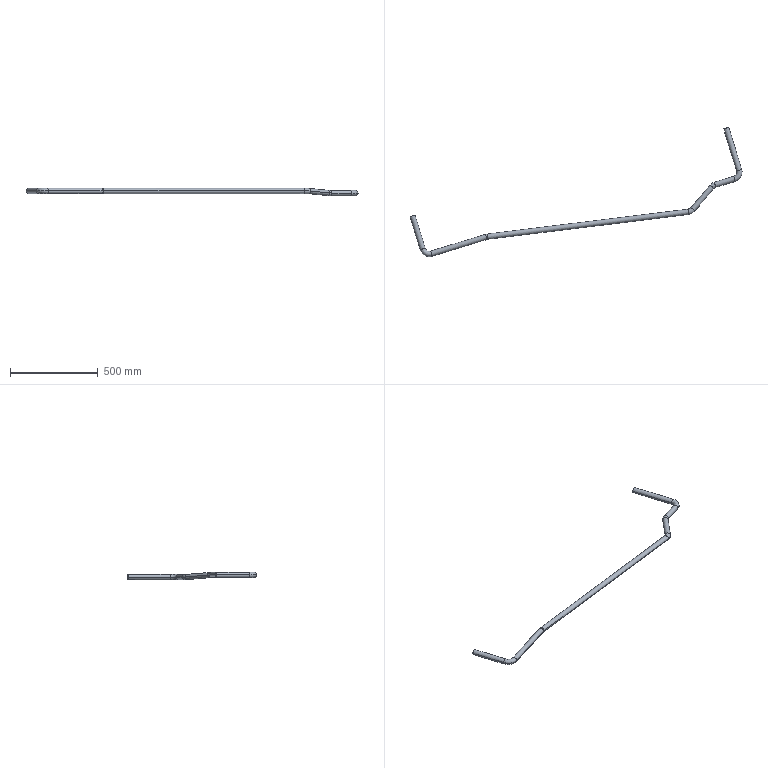Part | SolidWorks | features 3DProfileFeature 2, Sweep 1 | 1 solid | 46 faces | box 1894 x 737.142 x 42.475 mm | volume 941942 mm3 | cylinder 24 | torus 20 | plane 2 | commonest cylinder face diameters 20 x12 30 x12
STEP:
#1=CARTESIAN_POINT('',(1993.335,-11.562,-11.65));
#2=VERTEX_POINT('',#1);
#3=CARTESIAN_POINT('',(1999.193,-30.685,-11.65));
#4=VERTEX_POINT('',#3);
#5=CARTESIAN_POINT('',(1996.264,-21.124,-11.65));
#6=DIRECTION('',(-0.9561,-0.2929,0.));
#7=DIRECTION('',(-0.2929,0.9561,0.));
#8=AXIS2_PLACEMENT_3D('',#5,#6,#7);
#9=CIRCLE('',#8,10.);
#10=EDGE_CURVE('',#2,#4,#9,.T.);
#11=ORIENTED_EDGE('',*,*,#10,.T.);
#12=CARTESIAN_POINT('',(2032.355,31.767,-11.65));
#13=VERTEX_POINT('',#12);
#14=CARTESIAN_POINT('',(1984.548,17.122,-11.65));
#15=DIRECTION('',(0.,0.,1.));
#16=DIRECTION('',(0.,-1.,0.));
#17=AXIS2_PLACEMENT_3D('',#14,#15,#16);
#18=CIRCLE('',#17,50.);
#19=EDGE_CURVE('',#4,#13,#18,.T.);
#20=ORIENTED_EDGE('',*,*,#19,.T.);
#21=CARTESIAN_POINT('',(2013.232,25.909,-11.65));
#22=VERTEX_POINT('',#21);
#23=CARTESIAN_POINT('',(2022.793,28.838,-11.65));
#24=DIRECTION('',(0.2929,-0.9561,0.));
#25=DIRECTION('',(0.9561,0.2929,0.));
#26=AXIS2_PLACEMENT_3D('',#23,#24,#25);
#27=CIRCLE('',#26,10.);
#28=EDGE_CURVE('',#22,#13,#27,.T.);
#29=ORIENTED_EDGE('',*,*,#28,.F.);
#30=CARTESIAN_POINT('',(1984.548,17.122,-11.65));
#31=DIRECTION('',(0.,0.,1.));
#32=DIRECTION('',(0.,-1.,0.));
#33=AXIS2_PLACEMENT_3D('',#30,#31,#32);
#34=CIRCLE('',#33,30.);
#35=EDGE_CURVE('',#2,#22,#34,.T.);
#36=ORIENTED_EDGE('',*,*,#35,.F.);
#37=EDGE_LOOP('',(#11,#20,#29,#36));
#38=FACE_OUTER_BOUND('',#37,.T.);
#39=CARTESIAN_POINT('',(1984.548,17.122,-11.65));
#40=DIRECTION('',(0.,0.,1.));
#41=DIRECTION('',(0.,-1.,0.));
#42=AXIS2_PLACEMENT_3D('',#39,#40,#41);
#43=TOROIDAL_SURFACE('',#42,40.,10.);
#44=ADVANCED_FACE('',(#38),#43,.F.);
#45=CARTESIAN_POINT('',(1859.636,-60.808,-10.9));
#46=VERTEX_POINT('',#45);
#47=CARTESIAN_POINT('',(1859.633,-60.888,-11.886));
#48=VERTEX_POINT('',#47);
#49=CARTESIAN_POINT('',(1867.261,-67.278,-10.9));
#50=DIRECTION('',(-0.6457,-0.7609,0.06365));
#51=DIRECTION('',(-0.7625,0.647,0.));
#52=AXIS2_PLACEMENT_3D('',#49,#50,#51);
#53=CIRCLE('',#52,10.);
#54=EDGE_CURVE('',#46,#48,#53,.T.);
#55=ORIENTED_EDGE('',*,*,#54,.T.);
#56=CARTESIAN_POINT('',(1883.229,-45.365,-12.824));
#57=VERTEX_POINT('',#56);
#58=CARTESIAN_POINT('',(1897.773,-92.841,-6.953));
#59=DIRECTION('',(0.03439,-0.1123,-0.9931));
#60=DIRECTION('',(0.,0.9937,-0.1123));
#61=AXIS2_PLACEMENT_3D('',#58,#59,#60);
#62=CIRCLE('',#61,50.);
#63=EDGE_CURVE('',#48,#57,#62,.T.);
#64=ORIENTED_EDGE('',*,*,#63,.T.);
#65=CARTESIAN_POINT('',(1883.209,-45.298,-11.65));
#66=VERTEX_POINT('',#65);
#67=CARTESIAN_POINT('',(1886.138,-54.86,-11.65));
#68=DIRECTION('',(-0.9561,-0.2929,0.));
#69=DIRECTION('',(0.2929,-0.9561,0.));
#70=AXIS2_PLACEMENT_3D('',#67,#68,#69);
#71=CIRCLE('',#70,10.);
#72=EDGE_CURVE('',#66,#57,#71,.T.);
#73=ORIENTED_EDGE('',*,*,#72,.F.);
#74=CARTESIAN_POINT('',(1889.047,-64.355,-10.476));
#75=VERTEX_POINT('',#74);
#76=CARTESIAN_POINT('',(1886.138,-54.86,-11.65));
#77=DIRECTION('',(-0.9561,-0.2929,0.));
#78=DIRECTION('',(0.2929,-0.9561,0.));
#79=AXIS2_PLACEMENT_3D('',#76,#77,#78);
#80=CIRCLE('',#79,10.);
#81=EDGE_CURVE('',#75,#66,#80,.T.);
#82=ORIENTED_EDGE('',*,*,#81,.F.);
#83=CARTESIAN_POINT('',(1874.889,-73.669,-9.913));
#84=VERTEX_POINT('',#83);
#85=CARTESIAN_POINT('',(1897.773,-92.841,-6.953));
#86=DIRECTION('',(0.03439,-0.1123,-0.9931));
#87=DIRECTION('',(0.,0.9937,-0.1123));
#88=AXIS2_PLACEMENT_3D('',#85,#86,#87);
#89=CIRCLE('',#88,30.);
#90=EDGE_CURVE('',#84,#75,#89,.T.);
#91=ORIENTED_EDGE('',*,*,#90,.F.);
#92=CARTESIAN_POINT('',(1867.261,-67.278,-10.9));
#93=DIRECTION('',(-0.6457,-0.7609,0.06365));
#94=DIRECTION('',(-0.7625,0.647,0.));
#95=AXIS2_PLACEMENT_3D('',#92,#93,#94);
#96=CIRCLE('',#95,10.);
#97=EDGE_CURVE('',#84,#46,#96,.T.);
#98=ORIENTED_EDGE('',*,*,#97,.T.);
#99=EDGE_LOOP('',(#55,#64,#73,#82,#91,#98));
#100=FACE_OUTER_BOUND('',#99,.T.);
#101=CARTESIAN_POINT('',(1897.773,-92.841,-6.953));
#102=DIRECTION('',(0.03439,-0.1123,-0.9931));
#103=DIRECTION('',(0.,0.9937,-0.1123));
#104=AXIS2_PLACEMENT_3D('',#101,#102,#103);
#105=TOROIDAL_SURFACE('',#104,40.,10.);
#106=ADVANCED_FACE('',(#100),#105,.F.);
#107=CARTESIAN_POINT('',(1733.998,-219.279,0.8251));
#108=VERTEX_POINT('',#107);
#109=CARTESIAN_POINT('',(1733.992,-219.235,1.762));
#110=VERTEX_POINT('',#109);
#111=CARTESIAN_POINT('',(1732.773,-209.354,0.8251));
#112=DIRECTION('',(-0.9925,-0.1224,0.));
#113=DIRECTION('',(-0.1224,0.9925,0.));
#114=AXIS2_PLACEMENT_3D('',#111,#112,#113);
#115=CIRCLE('',#114,10.);
#116=EDGE_CURVE('',#108,#110,#115,.T.);
#117=ORIENTED_EDGE('',*,*,#116,.T.);
#118=CARTESIAN_POINT('',(1766.072,-201.937,0.5159));
#119=VERTEX_POINT('',#118);
#120=CARTESIAN_POINT('',(1727.898,-169.83,-2.924));
#121=DIRECTION('',(-0.01147,0.09302,0.9956));
#122=DIRECTION('',(0.,-0.9957,0.09303));
#123=AXIS2_PLACEMENT_3D('',#120,#121,#122);
#124=CIRCLE('',#123,50.);
#125=EDGE_CURVE('',#110,#119,#124,.T.);
#126=ORIENTED_EDGE('',*,*,#125,.T.);
#127=CARTESIAN_POINT('',(1766.062,-201.986,-0.1721));
#128=VERTEX_POINT('',#127);
#129=CARTESIAN_POINT('',(1758.438,-195.515,-0.1721));
#130=DIRECTION('',(-0.6457,-0.7609,0.06365));
#131=DIRECTION('',(0.7625,-0.647,0.));
#132=AXIS2_PLACEMENT_3D('',#129,#130,#131);
#133=CIRCLE('',#132,10.);
#134=EDGE_CURVE('',#128,#119,#133,.T.);
#135=ORIENTED_EDGE('',*,*,#134,.F.);
#136=CARTESIAN_POINT('',(1750.803,-189.094,-0.8601));
#137=VERTEX_POINT('',#136);
#138=CARTESIAN_POINT('',(1758.438,-195.515,-0.1721));
#139=DIRECTION('',(-0.6457,-0.7609,0.06365));
#140=DIRECTION('',(0.7625,-0.647,0.));
#141=AXIS2_PLACEMENT_3D('',#138,#139,#140);
#142=CIRCLE('',#141,10.);
#143=EDGE_CURVE('',#137,#128,#142,.T.);
#144=ORIENTED_EDGE('',*,*,#143,.F.);
#145=CARTESIAN_POINT('',(1731.555,-199.473,-0.1122));
#146=VERTEX_POINT('',#145);
#147=CARTESIAN_POINT('',(1727.898,-169.83,-2.924));
#148=DIRECTION('',(-0.01147,0.09302,0.9956));
#149=DIRECTION('',(0.,-0.9957,0.09303));
#150=AXIS2_PLACEMENT_3D('',#147,#148,#149);
#151=CIRCLE('',#150,30.);
#152=EDGE_CURVE('',#146,#137,#151,.T.);
#153=ORIENTED_EDGE('',*,*,#152,.F.);
#154=CARTESIAN_POINT('',(1732.773,-209.354,0.8251));
#155=DIRECTION('',(-0.9925,-0.1224,0.));
#156=DIRECTION('',(-0.1224,0.9925,0.));
#157=AXIS2_PLACEMENT_3D('',#154,#155,#156);
#158=CIRCLE('',#157,10.);
#159=EDGE_CURVE('',#146,#108,#158,.T.);
#160=ORIENTED_EDGE('',*,*,#159,.T.);
#161=EDGE_LOOP('',(#117,#126,#135,#144,#153,#160));
#162=FACE_OUTER_BOUND('',#161,.T.);
#163=CARTESIAN_POINT('',(1727.898,-169.83,-2.924));
#164=DIRECTION('',(-0.01147,0.09302,0.9956));
#165=DIRECTION('',(0.,-0.9957,0.09303));
#166=AXIS2_PLACEMENT_3D('',#163,#164,#165);
#167=TOROIDAL_SURFACE('',#166,40.,10.);
#168=ADVANCED_FACE('',(#162),#167,.F.);
#169=CARTESIAN_POINT('',(583.508,-361.652,0.8251));
#170=VERTEX_POINT('',#169);
#171=CARTESIAN_POINT('',(577.65,-342.529,0.8251));
#172=VERTEX_POINT('',#171);
#173=CARTESIAN_POINT('',(580.579,-352.09,0.8251));
#174=DIRECTION('',(-0.9561,-0.2929,0.));
#175=DIRECTION('',(-0.2929,0.9561,0.));
#176=AXIS2_PLACEMENT_3D('',#173,#174,#175);
#177=CIRCLE('',#176,10.);
#178=EDGE_CURVE('',#170,#172,#177,.T.);
#179=ORIENTED_EDGE('',*,*,#178,.T.);
#180=CARTESIAN_POINT('',(586.174,-340.712,0.8251));
#181=VERTEX_POINT('',#180);
#182=CARTESIAN_POINT('',(592.295,-390.336,0.8251));
#183=DIRECTION('',(0.,0.,-1.));
#184=DIRECTION('',(0.,1.,0.));
#185=AXIS2_PLACEMENT_3D('',#182,#183,#184);
#186=CIRCLE('',#185,50.);
#187=EDGE_CURVE('',#172,#181,#186,.T.);
#188=ORIENTED_EDGE('',*,*,#187,.T.);
#189=CARTESIAN_POINT('',(588.622,-360.561,0.8251));
#190=VERTEX_POINT('',#189);
#191=CARTESIAN_POINT('',(587.398,-350.637,0.8251));
#192=DIRECTION('',(-0.9925,-0.1224,0.));
#193=DIRECTION('',(0.1224,-0.9925,0.));
#194=AXIS2_PLACEMENT_3D('',#191,#192,#193);
#195=CIRCLE('',#194,10.);
#196=EDGE_CURVE('',#190,#181,#195,.T.);
#197=ORIENTED_EDGE('',*,*,#196,.F.);
#198=CARTESIAN_POINT('',(592.295,-390.336,0.8251));
#199=DIRECTION('',(0.,0.,-1.));
#200=DIRECTION('',(0.,1.,0.));
#201=AXIS2_PLACEMENT_3D('',#198,#199,#200);
#202=CIRCLE('',#201,30.);
#203=EDGE_CURVE('',#170,#190,#202,.T.);
#204=ORIENTED_EDGE('',*,*,#203,.F.);
#205=EDGE_LOOP('',(#179,#188,#197,#204));
#206=FACE_OUTER_BOUND('',#205,.T.);
#207=CARTESIAN_POINT('',(592.295,-390.336,0.8251));
#208=DIRECTION('',(0.,0.,-1.));
#209=DIRECTION('',(0.,1.,0.));
#210=AXIS2_PLACEMENT_3D('',#207,#208,#209);
#211=TOROIDAL_SURFACE('',#210,40.,10.);
#212=ADVANCED_FACE('',(#206),#211,.F.);
#213=CARTESIAN_POINT('',(227.44,-418.436,0.8251));
#214=VERTEX_POINT('',#213);
#215=CARTESIAN_POINT('',(208.318,-424.294,0.8251));
#216=VERTEX_POINT('',#215);
#217=CARTESIAN_POINT('',(217.879,-421.365,0.8251));
#218=DIRECTION('',(-0.2929,0.9561,0.));
#219=DIRECTION('',(0.9561,0.2929,0.));
#220=AXIS2_PLACEMENT_3D('',#217,#218,#219);
#221=CIRCLE('',#220,10.);
#222=EDGE_CURVE('',#214,#216,#221,.T.);
#223=ORIENTED_EDGE('',*,*,#222,.T.);
#224=CARTESIAN_POINT('',(270.77,-457.456,0.8251));
#225=VERTEX_POINT('',#224);
#226=CARTESIAN_POINT('',(256.125,-409.649,0.8251));
#227=DIRECTION('',(0.,0.,1.));
#228=DIRECTION('',(1.,0.,0.));
#229=AXIS2_PLACEMENT_3D('',#226,#227,#228);
#230=CIRCLE('',#229,50.);
#231=EDGE_CURVE('',#216,#225,#230,.T.);
#232=ORIENTED_EDGE('',*,*,#231,.T.);
#233=CARTESIAN_POINT('',(264.912,-438.333,0.8251));
#234=VERTEX_POINT('',#233);
#235=CARTESIAN_POINT('',(267.841,-447.894,0.8251));
#236=DIRECTION('',(-0.9561,-0.2929,0.));
#237=DIRECTION('',(0.2929,-0.9561,0.));
#238=AXIS2_PLACEMENT_3D('',#235,#236,#237);
#239=CIRCLE('',#238,10.);
#240=EDGE_CURVE('',#234,#225,#239,.T.);
#241=ORIENTED_EDGE('',*,*,#240,.F.);
#242=CARTESIAN_POINT('',(256.125,-409.649,0.8251));
#243=DIRECTION('',(0.,0.,1.));
#244=DIRECTION('',(1.,0.,0.));
#245=AXIS2_PLACEMENT_3D('',#242,#243,#244);
#246=CIRCLE('',#245,30.);
#247=EDGE_CURVE('',#214,#234,#246,.T.);
#248=ORIENTED_EDGE('',*,*,#247,.F.);
#249=EDGE_LOOP('',(#223,#232,#241,#248));
#250=FACE_OUTER_BOUND('',#249,.T.);
#251=CARTESIAN_POINT('',(256.125,-409.649,0.8251));
#252=DIRECTION('',(0.,0.,1.));
#253=DIRECTION('',(1.,0.,0.));
#254=AXIS2_PLACEMENT_3D('',#251,#252,#253);
#255=TOROIDAL_SURFACE('',#254,40.,10.);
#256=ADVANCED_FACE('',(#250),#255,.F.);
#257=CARTESIAN_POINT('',(2000.658,-35.466,-11.65));
#258=VERTEX_POINT('',#257);
#259=CARTESIAN_POINT('',(1991.87,-6.782,-11.65));
#260=VERTEX_POINT('',#259);
#261=CARTESIAN_POINT('',(1996.264,-21.124,-11.65));
#262=DIRECTION('',(-0.9561,-0.2929,0.));
#263=DIRECTION('',(0.2929,-0.9561,0.));
#264=AXIS2_PLACEMENT_3D('',#261,#262,#263);
#265=CIRCLE('',#264,15.);
#266=EDGE_CURVE('',#258,#260,#265,.T.);
#267=ORIENTED_EDGE('',*,*,#266,.F.);
#268=CARTESIAN_POINT('',(2037.136,33.232,-11.65));
#269=VERTEX_POINT('',#268);
#270=CARTESIAN_POINT('',(1984.548,17.122,-11.65));
#271=DIRECTION('',(0.,0.,1.));
#272=DIRECTION('',(0.,-1.,0.));
#273=AXIS2_PLACEMENT_3D('',#270,#271,#272);
#274=CIRCLE('',#273,55.);
#275=EDGE_CURVE('',#258,#269,#274,.T.);
#276=ORIENTED_EDGE('',*,*,#275,.T.);
#277=CARTESIAN_POINT('',(2008.451,24.445,-11.65));
#278=VERTEX_POINT('',#277);
#279=CARTESIAN_POINT('',(2022.793,28.838,-11.65));
#280=DIRECTION('',(0.2929,-0.9561,0.));
#281=DIRECTION('',(0.9561,0.2929,0.));
#282=AXIS2_PLACEMENT_3D('',#279,#280,#281);
#283=CIRCLE('',#282,15.);
#284=EDGE_CURVE('',#269,#278,#283,.T.);
#285=ORIENTED_EDGE('',*,*,#284,.T.);
#286=CARTESIAN_POINT('',(1984.548,17.122,-11.65));
#287=DIRECTION('',(0.,0.,1.));
#288=DIRECTION('',(0.,-1.,0.));
#289=AXIS2_PLACEMENT_3D('',#286,#287,#288);
#290=CIRCLE('',#289,25.);
#291=EDGE_CURVE('',#260,#278,#290,.T.);
#292=ORIENTED_EDGE('',*,*,#291,.F.);
#293=EDGE_LOOP('',(#267,#276,#285,#292));
#294=FACE_OUTER_BOUND('',#293,.T.);
#295=CARTESIAN_POINT('',(1984.548,17.122,-11.65));
#296=DIRECTION('',(0.,0.,1.));
#297=DIRECTION('',(0.,-1.,0.));
#298=AXIS2_PLACEMENT_3D('',#295,#296,#297);
#299=TOROIDAL_SURFACE('',#298,40.,15.);
#300=ADVANCED_FACE('',(#294),#299,.T.);
#301=CARTESIAN_POINT('',(1855.819,-57.692,-12.379));
#302=VERTEX_POINT('',#301);
#303=CARTESIAN_POINT('',(1878.698,-76.984,-10.9));
#304=VERTEX_POINT('',#303);
#305=CARTESIAN_POINT('',(1867.261,-67.278,-10.9));
#306=DIRECTION('',(-0.6457,-0.7609,0.06365));
#307=DIRECTION('',(0.7616,-0.6478,-0.01862));
#308=AXIS2_PLACEMENT_3D('',#305,#306,#307);
#309=CIRCLE('',#308,15.);
#310=EDGE_CURVE('',#302,#304,#309,.T.);
#311=ORIENTED_EDGE('',*,*,#310,.F.);
#312=CARTESIAN_POINT('',(1881.775,-40.617,-13.411));
#313=VERTEX_POINT('',#312);
#314=CARTESIAN_POINT('',(1897.773,-92.841,-6.953));
#315=DIRECTION('',(0.03439,-0.1123,-0.9931));
#316=DIRECTION('',(0.,0.9937,-0.1123));
#317=AXIS2_PLACEMENT_3D('',#314,#315,#316);
#318=CIRCLE('',#317,55.);
#319=EDGE_CURVE('',#302,#313,#318,.T.);
#320=ORIENTED_EDGE('',*,*,#319,.T.);
#321=CARTESIAN_POINT('',(1890.531,-69.202,-11.65));
#322=VERTEX_POINT('',#321);
#323=CARTESIAN_POINT('',(1886.138,-54.86,-11.65));
#324=DIRECTION('',(-0.9561,-0.2929,0.));
#325=DIRECTION('',(0.2929,-0.9561,0.));
#326=AXIS2_PLACEMENT_3D('',#323,#324,#325);
#327=CIRCLE('',#326,15.);
#328=EDGE_CURVE('',#313,#322,#327,.T.);
#329=ORIENTED_EDGE('',*,*,#328,.T.);
#330=CARTESIAN_POINT('',(1890.501,-69.103,-9.889));
#331=VERTEX_POINT('',#330);
#332=CARTESIAN_POINT('',(1886.138,-54.86,-11.65));
#333=DIRECTION('',(-0.9561,-0.2929,0.));
#334=DIRECTION('',(0.2929,-0.9561,0.));
#335=AXIS2_PLACEMENT_3D('',#332,#333,#334);
#336=CIRCLE('',#335,15.);
#337=EDGE_CURVE('',#322,#331,#336,.T.);
#338=ORIENTED_EDGE('',*,*,#337,.T.);
#339=CARTESIAN_POINT('',(1878.703,-76.864,-9.42));
#340=VERTEX_POINT('',#339);
#341=CARTESIAN_POINT('',(1897.773,-92.841,-6.953));
#342=DIRECTION('',(0.03439,-0.1123,-0.9931));
#343=DIRECTION('',(0.,0.9937,-0.1123));
#344=AXIS2_PLACEMENT_3D('',#341,#342,#343);
#345=CIRCLE('',#344,25.);
#346=EDGE_CURVE('',#340,#331,#345,.T.);
#347=ORIENTED_EDGE('',*,*,#346,.F.);
#348=CARTESIAN_POINT('',(1867.261,-67.278,-10.9));
#349=DIRECTION('',(-0.6457,-0.7609,0.06365));
#350=DIRECTION('',(0.7616,-0.6478,-0.01862));
#351=AXIS2_PLACEMENT_3D('',#348,#349,#350);
#352=CIRCLE('',#351,15.);
#353=EDGE_CURVE('',#304,#340,#352,.T.);
#354=ORIENTED_EDGE('',*,*,#353,.F.);
#355=EDGE_LOOP('',(#311,#320,#329,#338,#347,#354));
#356=FACE_OUTER_BOUND('',#355,.T.);
#357=CARTESIAN_POINT('',(1897.773,-92.841,-6.953));
#358=DIRECTION('',(0.03439,-0.1123,-0.9931));
#359=DIRECTION('',(0.,0.9937,-0.1123));
#360=AXIS2_PLACEMENT_3D('',#357,#358,#359);
#361=TOROIDAL_SURFACE('',#360,40.,15.);
#362=ADVANCED_FACE('',(#356),#361,.T.);
#363=CARTESIAN_POINT('',(1734.602,-224.176,2.231));
#364=VERTEX_POINT('',#363);
#365=CARTESIAN_POINT('',(1730.937,-194.467,0.8251));
#366=VERTEX_POINT('',#365);
#367=CARTESIAN_POINT('',(1732.773,-209.354,0.8251));
#368=DIRECTION('',(-0.9925,-0.1224,0.));
#369=DIRECTION('',(0.1224,-0.9925,0.006211));
#370=AXIS2_PLACEMENT_3D('',#367,#368,#369);
#371=CIRCLE('',#370,15.);
#372=EDGE_CURVE('',#364,#366,#371,.T.);
#373=ORIENTED_EDGE('',*,*,#372,.F.);
#374=CARTESIAN_POINT('',(1769.89,-205.148,0.8598));
#375=VERTEX_POINT('',#374);
#376=CARTESIAN_POINT('',(1727.898,-169.83,-2.924));
#377=DIRECTION('',(-0.01147,0.09302,0.9956));
#378=DIRECTION('',(0.,-0.9957,0.09303));
#379=AXIS2_PLACEMENT_3D('',#376,#377,#378);
#380=CIRCLE('',#379,55.);
#381=EDGE_CURVE('',#364,#375,#380,.T.);
#382=ORIENTED_EDGE('',*,*,#381,.T.);
#383=CARTESIAN_POINT('',(1747.001,-185.81,-0.1721));
#384=VERTEX_POINT('',#383);
#385=CARTESIAN_POINT('',(1758.438,-195.515,-0.1721));
#386=DIRECTION('',(-0.6457,-0.7609,0.06365));
#387=DIRECTION('',(0.7616,-0.6478,-0.01862));
#388=AXIS2_PLACEMENT_3D('',#385,#386,#387);
#389=CIRCLE('',#388,15.);
#390=EDGE_CURVE('',#375,#384,#389,.T.);
#391=ORIENTED_EDGE('',*,*,#390,.T.);
#392=CARTESIAN_POINT('',(1746.985,-185.883,-1.204));
#393=VERTEX_POINT('',#392);
#394=CARTESIAN_POINT('',(1758.438,-195.515,-0.1721));
#395=DIRECTION('',(-0.6457,-0.7609,0.06365));
#396=DIRECTION('',(0.7616,-0.6478,-0.01862));
#397=AXIS2_PLACEMENT_3D('',#394,#395,#396);
#398=CIRCLE('',#397,15.);
#399=EDGE_CURVE('',#384,#393,#398,.T.);
#400=ORIENTED_EDGE('',*,*,#399,.T.);
#401=CARTESIAN_POINT('',(1730.945,-194.532,-0.5808));
#402=VERTEX_POINT('',#401);
#403=CARTESIAN_POINT('',(1727.898,-169.83,-2.924));
#404=DIRECTION('',(-0.01147,0.09302,0.9956));
#405=DIRECTION('',(0.,-0.9957,0.09303));
#406=AXIS2_PLACEMENT_3D('',#403,#404,#405);
#407=CIRCLE('',#406,25.);
#408=EDGE_CURVE('',#402,#393,#407,.T.);
#409=ORIENTED_EDGE('',*,*,#408,.F.);
#410=CARTESIAN_POINT('',(1732.773,-209.354,0.8251));
#411=DIRECTION('',(-0.9925,-0.1224,0.));
#412=DIRECTION('',(0.1224,-0.9925,0.006211));
#413=AXIS2_PLACEMENT_3D('',#410,#411,#412);
#414=CIRCLE('',#413,15.);
#415=EDGE_CURVE('',#366,#402,#414,.T.);
#416=ORIENTED_EDGE('',*,*,#415,.F.);
#417=EDGE_LOOP('',(#373,#382,#391,#400,#409,#416));
#418=FACE_OUTER_BOUND('',#417,.T.);
#419=CARTESIAN_POINT('',(1727.898,-169.83,-2.924));
#420=DIRECTION('',(-0.01147,0.09302,0.9956));
#421=DIRECTION('',(0.,-0.9957,0.09303));
#422=AXIS2_PLACEMENT_3D('',#419,#420,#421);
#423=TOROIDAL_SURFACE('',#422,40.,15.);
#424=ADVANCED_FACE('',(#418),#423,.T.);
#425=CARTESIAN_POINT('',(576.185,-337.748,0.8251));
#426=VERTEX_POINT('',#425);
#427=CARTESIAN_POINT('',(584.973,-366.432,0.8251));
#428=VERTEX_POINT('',#427);
#429=CARTESIAN_POINT('',(580.579,-352.09,0.8251));
#430=DIRECTION('',(-0.9561,-0.2929,0.));
#431=DIRECTION('',(0.2929,-0.9561,0.006211));
#432=AXIS2_PLACEMENT_3D('',#429,#430,#431);
#433=CIRCLE('',#432,15.);
#434=EDGE_CURVE('',#426,#428,#433,.T.);
#435=ORIENTED_EDGE('',*,*,#434,.F.);
#436=CARTESIAN_POINT('',(585.562,-335.749,0.8251));
#437=VERTEX_POINT('',#436);
#438=CARTESIAN_POINT('',(592.295,-390.336,0.8251));
#439=DIRECTION('',(0.,0.,-1.));
#440=DIRECTION('',(0.,1.,0.));
#441=AXIS2_PLACEMENT_3D('',#438,#439,#440);
#442=CIRCLE('',#441,55.);
#443=EDGE_CURVE('',#426,#437,#442,.T.);
#444=ORIENTED_EDGE('',*,*,#443,.T.);
#445=CARTESIAN_POINT('',(589.235,-365.524,0.8251));
#446=VERTEX_POINT('',#445);
#447=CARTESIAN_POINT('',(587.398,-350.637,0.8251));
#448=DIRECTION('',(-0.9925,-0.1224,0.));
#449=DIRECTION('',(0.1224,-0.9925,0.006211));
#450=AXIS2_PLACEMENT_3D('',#447,#448,#449);
#451=CIRCLE('',#450,15.);
#452=EDGE_CURVE('',#437,#446,#451,.T.);
#453=ORIENTED_EDGE('',*,*,#452,.T.);
#454=CARTESIAN_POINT('',(592.295,-390.336,0.8251));
#455=DIRECTION('',(0.,0.,-1.));
#456=DIRECTION('',(0.,1.,0.));
#457=AXIS2_PLACEMENT_3D('',#454,#455,#456);
#458=CIRCLE('',#457,25.);
#459=EDGE_CURVE('',#428,#446,#458,.T.);
#460=ORIENTED_EDGE('',*,*,#459,.F.);
#461=EDGE_LOOP('',(#435,#444,#453,#460));
#462=FACE_OUTER_BOUND('',#461,.T.);
#463=CARTESIAN_POINT('',(592.295,-390.336,0.8251));
#464=DIRECTION('',(0.,0.,-1.));
#465=DIRECTION('',(0.,1.,0.));
#466=AXIS2_PLACEMENT_3D('',#463,#464,#465);
#467=TOROIDAL_SURFACE('',#466,40.,15.);
#468=ADVANCED_FACE('',(#462),#467,.T.);
#469=CARTESIAN_POINT('',(203.537,-425.759,0.8251));
#470=VERTEX_POINT('',#469);
#471=CARTESIAN_POINT('',(232.221,-416.971,0.8251));
#472=VERTEX_POINT('',#471);
#473=CARTESIAN_POINT('',(217.879,-421.365,0.8251));
#474=DIRECTION('',(-0.2929,0.9561,0.));
#475=DIRECTION('',(-0.9561,-0.2929,0.006211));
#476=AXIS2_PLACEMENT_3D('',#473,#474,#475);
#477=CIRCLE('',#476,15.);
#478=EDGE_CURVE('',#470,#472,#477,.T.);
#479=ORIENTED_EDGE('',*,*,#478,.F.);
#480=CARTESIAN_POINT('',(272.234,-462.237,0.8251));
#481=VERTEX_POINT('',#480);
#482=CARTESIAN_POINT('',(256.125,-409.649,0.8251));
#483=DIRECTION('',(0.,0.,1.));
#484=DIRECTION('',(1.,0.,0.));
#485=AXIS2_PLACEMENT_3D('',#482,#483,#484);
#486=CIRCLE('',#485,55.);
#487=EDGE_CURVE('',#470,#481,#486,.T.);
#488=ORIENTED_EDGE('',*,*,#487,.T.);
#489=CARTESIAN_POINT('',(263.447,-433.552,0.8251));
#490=VERTEX_POINT('',#489);
#491=CARTESIAN_POINT('',(267.841,-447.894,0.8251));
#492=DIRECTION('',(-0.9561,-0.2929,0.));
#493=DIRECTION('',(0.2929,-0.9561,0.006211));
#494=AXIS2_PLACEMENT_3D('',#491,#492,#493);
#495=CIRCLE('',#494,15.);
#496=EDGE_CURVE('',#481,#490,#495,.T.);
#497=ORIENTED_EDGE('',*,*,#496,.T.);
#498=CARTESIAN_POINT('',(256.125,-409.649,0.8251));
#499=DIRECTION('',(0.,0.,1.));
#500=DIRECTION('',(1.,0.,0.));
#501=AXIS2_PLACEMENT_3D('',#498,#499,#500);
#502=CIRCLE('',#501,25.);
#503=EDGE_CURVE('',#472,#490,#502,.T.);
#504=ORIENTED_EDGE('',*,*,#503,.F.);
#505=EDGE_LOOP('',(#479,#488,#497,#504));
#506=FACE_OUTER_BOUND('',#505,.T.);
#507=CARTESIAN_POINT('',(256.125,-409.649,0.8251));
#508=DIRECTION('',(0.,0.,1.));
#509=DIRECTION('',(1.,0.,0.));
#510=AXIS2_PLACEMENT_3D('',#507,#508,#509);
#511=TOROIDAL_SURFACE('',#510,40.,15.);
#512=ADVANCED_FACE('',(#506),#511,.T.);
#513=ORIENTED_EDGE('',*,*,#28,.T.);
#514=CARTESIAN_POINT('',(1959.059,271.028,-11.65));
#515=VERTEX_POINT('',#514);
#516=CARTESIAN_POINT('',(2032.355,31.767,-11.65));
#517=DIRECTION('',(-0.2929,0.9561,0.));
#518=VECTOR('',#517,1000.);
#519=LINE('',#516,#518);
#520=EDGE_CURVE('',#13,#515,#519,.T.);
#521=ORIENTED_EDGE('',*,*,#520,.T.);
#522=CARTESIAN_POINT('',(1939.937,265.17,-11.65));
#523=VERTEX_POINT('',#522);
#524=CARTESIAN_POINT('',(1949.498,268.099,-11.65));
#525=DIRECTION('',(0.2929,-0.9561,0.));
#526=DIRECTION('',(0.9561,0.2929,0.));
#527=AXIS2_PLACEMENT_3D('',#524,#525,#526);
#528=CIRCLE('',#527,10.);
#529=EDGE_CURVE('',#523,#515,#528,.T.);
#530=ORIENTED_EDGE('',*,*,#529,.F.);
#531=CARTESIAN_POINT('',(2013.232,25.909,-11.65));
#532=DIRECTION('',(-0.2929,0.9561,0.));
#533=VECTOR('',#532,1000.);
#534=LINE('',#531,#533);
#535=EDGE_CURVE('',#22,#523,#534,.T.);
#536=ORIENTED_EDGE('',*,*,#535,.F.);
#537=EDGE_LOOP('',(#513,#521,#530,#536));
#538=FACE_OUTER_BOUND('',#537,.T.);
#539=CARTESIAN_POINT('',(2022.793,28.838,-11.65));
#540=DIRECTION('',(-0.2929,0.9561,0.));
#541=DIRECTION('',(-0.9561,-0.2929,0.));
#542=AXIS2_PLACEMENT_3D('',#539,#540,#541);
#543=CYLINDRICAL_SURFACE('',#542,10.);
#544=ADVANCED_FACE('',(#538),#543,.F.);
#545=ORIENTED_EDGE('',*,*,#72,.T.);
#546=CARTESIAN_POINT('',(1889.067,-64.421,-11.65));
#547=VERTEX_POINT('',#546);
#548=CARTESIAN_POINT('',(1886.138,-54.86,-11.65));
#549=DIRECTION('',(-0.9561,-0.2929,0.));
#550=DIRECTION('',(0.2929,-0.9561,0.));
#551=AXIS2_PLACEMENT_3D('',#548,#549,#550);
#552=CIRCLE('',#551,10.);
#553=EDGE_CURVE('',#57,#547,#552,.T.);
#554=ORIENTED_EDGE('',*,*,#553,.T.);
#555=CARTESIAN_POINT('',(1889.067,-64.421,-11.65));
#556=DIRECTION('',(0.9561,0.2929,0.));
#557=VECTOR('',#556,1000.);
#558=LINE('',#555,#557);
#559=EDGE_CURVE('',#547,#4,#558,.T.);
#560=ORIENTED_EDGE('',*,*,#559,.T.);
#561=ORIENTED_EDGE('',*,*,#10,.F.);
#562=CARTESIAN_POINT('',(1883.209,-45.298,-11.65));
#563=DIRECTION('',(0.9561,0.2929,0.));
#564=VECTOR('',#563,1000.);
#565=LINE('',#562,#564);
#566=EDGE_CURVE('',#66,#2,#565,.T.);
#567=ORIENTED_EDGE('',*,*,#566,.F.);
#568=EDGE_LOOP('',(#545,#554,#560,#561,#567));
#569=FACE_OUTER_BOUND('',#568,.T.);
#570=CARTESIAN_POINT('',(1886.138,-54.86,-11.65));
#571=DIRECTION('',(0.9561,0.2929,0.));
#572=DIRECTION('',(-0.2929,0.9561,0.));
#573=AXIS2_PLACEMENT_3D('',#570,#571,#572);
#574=CYLINDRICAL_SURFACE('',#573,10.);
#575=ADVANCED_FACE('',(#569),#574,.F.);
#576=CARTESIAN_POINT('',(1750.813,-189.045,-0.1721));
#577=VERTEX_POINT('',#576);
#578=CARTESIAN_POINT('',(1758.438,-195.515,-0.1721));
#579=DIRECTION('',(-0.6457,-0.7609,0.06365));
#580=DIRECTION('',(0.7625,-0.647,0.));
#581=AXIS2_PLACEMENT_3D('',#578,#579,#580);
#582=CIRCLE('',#581,10.);
#583=EDGE_CURVE('',#577,#137,#582,.T.);
#584=ORIENTED_EDGE('',*,*,#583,.T.);
#585=ORIENTED_EDGE('',*,*,#143,.T.);
#586=CARTESIAN_POINT('',(1874.886,-73.749,-10.9));
#587=VERTEX_POINT('',#586);
#588=CARTESIAN_POINT('',(1766.062,-201.986,-0.1721));
#589=DIRECTION('',(0.6457,0.7609,-0.06365));
#590=VECTOR('',#589,1000.);
#591=LINE('',#588,#590);
#592=EDGE_CURVE('',#128,#587,#591,.T.);
#593=ORIENTED_EDGE('',*,*,#592,.T.);
#594=CARTESIAN_POINT('',(1867.261,-67.278,-10.9));
#595=DIRECTION('',(-0.6457,-0.7609,0.06365));
#596=DIRECTION('',(-0.7625,0.647,0.));
#597=AXIS2_PLACEMENT_3D('',#594,#595,#596);
#598=CIRCLE('',#597,10.);
#599=EDGE_CURVE('',#48,#587,#598,.T.);
#600=ORIENTED_EDGE('',*,*,#599,.F.);
#601=ORIENTED_EDGE('',*,*,#54,.F.);
#602=CARTESIAN_POINT('',(1750.813,-189.045,-0.1721));
#603=DIRECTION('',(0.6457,0.7609,-0.06365));
#604=VECTOR('',#603,1000.);
#605=LINE('',#602,#604);
#606=EDGE_CURVE('',#577,#46,#605,.T.);
#607=ORIENTED_EDGE('',*,*,#606,.F.);
#608=EDGE_LOOP('',(#584,#585,#593,#600,#601,#607));
#609=FACE_OUTER_BOUND('',#608,.T.);
#610=CARTESIAN_POINT('',(1758.438,-195.515,-0.1721));
#611=DIRECTION('',(0.6457,0.7609,-0.06365));
#612=DIRECTION('',(-0.7625,0.647,0.));
#613=AXIS2_PLACEMENT_3D('',#610,#611,#612);
#614=CYLINDRICAL_SURFACE('',#613,10.);
#615=ADVANCED_FACE('',(#609),#614,.F.);
#616=CARTESIAN_POINT('',(587.398,-350.637,0.8251));
#617=DIRECTION('',(-0.9925,-0.1224,0.));
#618=DIRECTION('',(0.1224,-0.9925,0.));
#619=AXIS2_PLACEMENT_3D('',#616,#617,#618);
#620=CIRCLE('',#619,10.);
#621=EDGE_CURVE('',#181,#190,#620,.T.);
#622=ORIENTED_EDGE('',*,*,#621,.T.);
#623=CARTESIAN_POINT('',(588.622,-360.561,0.8251));
#624=DIRECTION('',(0.9925,0.1224,0.));
#625=VECTOR('',#624,1000.);
#626=LINE('',#623,#625);
#627=EDGE_CURVE('',#190,#108,#626,.T.);
#628=ORIENTED_EDGE('',*,*,#627,.T.);
#629=ORIENTED_EDGE('',*,*,#159,.F.);
#630=CARTESIAN_POINT('',(1731.549,-199.429,0.8251));
#631=VERTEX_POINT('',#630);
#632=CARTESIAN_POINT('',(1732.773,-209.354,0.8251));
#633=DIRECTION('',(-0.9925,-0.1224,0.));
#634=DIRECTION('',(-0.1224,0.9925,0.));
#635=AXIS2_PLACEMENT_3D('',#632,#633,#634);
#636=CIRCLE('',#635,10.);
#637=EDGE_CURVE('',#631,#146,#636,.T.);
#638=ORIENTED_EDGE('',*,*,#637,.F.);
#639=CARTESIAN_POINT('',(586.174,-340.712,0.8251));
#640=DIRECTION('',(0.9925,0.1224,0.));
#641=VECTOR('',#640,1000.);
#642=LINE('',#639,#641);
#643=EDGE_CURVE('',#181,#631,#642,.T.);
#644=ORIENTED_EDGE('',*,*,#643,.F.);
#645=EDGE_LOOP('',(#622,#628,#629,#638,#644));
#646=FACE_OUTER_BOUND('',#645,.T.);
#647=CARTESIAN_POINT('',(587.398,-350.637,0.8251));
#648=DIRECTION('',(0.9925,0.1224,0.));
#649=DIRECTION('',(-0.1224,0.9925,0.));
#650=AXIS2_PLACEMENT_3D('',#647,#648,#649);
#651=CYLINDRICAL_SURFACE('',#650,10.);
#652=ADVANCED_FACE('',(#646),#651,.F.);
#653=ORIENTED_EDGE('',*,*,#240,.T.);
#654=CARTESIAN_POINT('',(270.77,-457.456,0.8251));
#655=DIRECTION('',(0.9561,0.2929,0.));
#656=VECTOR('',#655,1000.);
#657=LINE('',#654,#656);
#658=EDGE_CURVE('',#225,#170,#657,.T.);
#659=ORIENTED_EDGE('',*,*,#658,.T.);
#660=CARTESIAN_POINT('',(580.579,-352.09,0.8251));
#661=DIRECTION('',(-0.9561,-0.2929,0.));
#662=DIRECTION('',(-0.2929,0.9561,0.));
#663=AXIS2_PLACEMENT_3D('',#660,#661,#662);
#664=CIRCLE('',#663,10.);
#665=EDGE_CURVE('',#172,#170,#664,.T.);
#666=ORIENTED_EDGE('',*,*,#665,.F.);
#667=CARTESIAN_POINT('',(264.912,-438.333,0.8251));
#668=DIRECTION('',(0.9561,0.2929,0.));
#669=VECTOR('',#668,1000.);
#670=LINE('',#667,#669);
#671=EDGE_CURVE('',#234,#172,#670,.T.);
#672=ORIENTED_EDGE('',*,*,#671,.F.);
#673=EDGE_LOOP('',(#653,#659,#666,#672));
#674=FACE_OUTER_BOUND('',#673,.T.);
#675=CARTESIAN_POINT('',(267.841,-447.894,0.8251));
#676=DIRECTION('',(0.9561,0.2929,0.));
#677=DIRECTION('',(-0.2929,0.9561,0.));
#678=AXIS2_PLACEMENT_3D('',#675,#676,#677);
#679=CYLINDRICAL_SURFACE('',#678,10.);
#680=ADVANCED_FACE('',(#674),#679,.F.);
#681=CARTESIAN_POINT('',(169.409,-229.002,0.8251));
#682=VERTEX_POINT('',#681);
#683=CARTESIAN_POINT('',(150.286,-234.86,0.8251));
#684=VERTEX_POINT('',#683);
#685=CARTESIAN_POINT('',(159.848,-231.931,0.8251));
#686=DIRECTION('',(-0.2929,0.9561,0.));
#687=DIRECTION('',(-0.9561,-0.2929,0.));
#688=AXIS2_PLACEMENT_3D('',#685,#686,#687);
#689=CIRCLE('',#688,10.);
#690=EDGE_CURVE('',#682,#684,#689,.T.);
#691=ORIENTED_EDGE('',*,*,#690,.T.);
#692=CARTESIAN_POINT('',(150.286,-234.86,0.8251));
#693=DIRECTION('',(0.2929,-0.9561,0.));
#694=VECTOR('',#693,1000.);
#695=LINE('',#692,#694);
#696=EDGE_CURVE('',#684,#216,#695,.T.);
#697=ORIENTED_EDGE('',*,*,#696,.T.);
#698=ORIENTED_EDGE('',*,*,#222,.F.);
#699=CARTESIAN_POINT('',(169.409,-229.002,0.8251));
#700=DIRECTION('',(0.2929,-0.9561,0.));
#701=VECTOR('',#700,1000.);
#702=LINE('',#699,#701);
#703=EDGE_CURVE('',#682,#214,#702,.T.);
#704=ORIENTED_EDGE('',*,*,#703,.F.);
#705=EDGE_LOOP('',(#691,#697,#698,#704));
#706=FACE_OUTER_BOUND('',#705,.T.);
#707=CARTESIAN_POINT('',(159.848,-231.931,0.8251));
#708=DIRECTION('',(0.2929,-0.9561,0.));
#709=DIRECTION('',(0.9561,0.2929,0.));
#710=AXIS2_PLACEMENT_3D('',#707,#708,#709);
#711=CYLINDRICAL_SURFACE('',#710,10.);
#712=ADVANCED_FACE('',(#706),#711,.F.);
#713=ORIENTED_EDGE('',*,*,#284,.F.);
#714=CARTESIAN_POINT('',(1963.84,272.493,-11.65));
#715=VERTEX_POINT('',#714);
#716=CARTESIAN_POINT('',(2037.136,33.232,-11.65));
#717=DIRECTION('',(-0.2929,0.9561,0.));
#718=VECTOR('',#717,1000.);
#719=LINE('',#716,#718);
#720=EDGE_CURVE('',#269,#715,#719,.T.);
#721=ORIENTED_EDGE('',*,*,#720,.T.);
#722=CARTESIAN_POINT('',(1935.156,263.706,-11.65));
#723=VERTEX_POINT('',#722);
#724=CARTESIAN_POINT('',(1949.498,268.099,-11.65));
#725=DIRECTION('',(0.2929,-0.9561,0.));
#726=DIRECTION('',(0.9561,0.2929,0.));
#727=AXIS2_PLACEMENT_3D('',#724,#725,#726);
#728=CIRCLE('',#727,15.);
#729=EDGE_CURVE('',#715,#723,#728,.T.);
#730=ORIENTED_EDGE('',*,*,#729,.T.);
#731=CARTESIAN_POINT('',(2008.451,24.445,-11.65));
#732=DIRECTION('',(-0.2929,0.9561,0.));
#733=VECTOR('',#732,1000.);
#734=LINE('',#731,#733);
#735=EDGE_CURVE('',#278,#723,#734,.T.);
#736=ORIENTED_EDGE('',*,*,#735,.F.);
#737=EDGE_LOOP('',(#713,#721,#730,#736));
#738=FACE_OUTER_BOUND('',#737,.T.);
#739=CARTESIAN_POINT('',(2022.793,28.838,-11.65));
#740=DIRECTION('',(-0.2929,0.9561,0.));
#741=DIRECTION('',(-0.9561,-0.2929,0.));
#742=AXIS2_PLACEMENT_3D('',#739,#740,#741);
#743=CYLINDRICAL_SURFACE('',#742,15.);
#744=ADVANCED_FACE('',(#738),#743,.T.);
#745=ORIENTED_EDGE('',*,*,#337,.F.);
#746=CARTESIAN_POINT('',(1890.531,-69.202,-11.65));
#747=DIRECTION('',(0.9561,0.2929,0.));
#748=VECTOR('',#747,1000.);
#749=LINE('',#746,#748);
#750=EDGE_CURVE('',#322,#258,#749,.T.);
#751=ORIENTED_EDGE('',*,*,#750,.T.);
#752=ORIENTED_EDGE('',*,*,#266,.T.);
#753=CARTESIAN_POINT('',(1881.744,-40.518,-11.65));
#754=VERTEX_POINT('',#753);
#755=CARTESIAN_POINT('',(1881.744,-40.518,-11.65));
#756=DIRECTION('',(0.9561,0.2929,0.));
#757=VECTOR('',#756,1000.);
#758=LINE('',#755,#757);
#759=EDGE_CURVE('',#754,#260,#758,.T.);
#760=ORIENTED_EDGE('',*,*,#759,.F.);
#761=CARTESIAN_POINT('',(1886.138,-54.86,-11.65));
#762=DIRECTION('',(-0.9561,-0.2929,0.));
#763=DIRECTION('',(0.2929,-0.9561,0.));
#764=AXIS2_PLACEMENT_3D('',#761,#762,#763);
#765=CIRCLE('',#764,15.);
#766=EDGE_CURVE('',#331,#754,#765,.T.);
#767=ORIENTED_EDGE('',*,*,#766,.F.);
#768=EDGE_LOOP('',(#745,#751,#752,#760,#767));
#769=FACE_OUTER_BOUND('',#768,.T.);
#770=CARTESIAN_POINT('',(1886.138,-54.86,-11.65));
#771=DIRECTION('',(0.9561,0.2929,0.));
#772=DIRECTION('',(-0.2929,0.9561,0.));
#773=AXIS2_PLACEMENT_3D('',#770,#771,#772);
#774=CYLINDRICAL_SURFACE('',#773,15.);
#775=ADVANCED_FACE('',(#769),#774,.T.);
#776=CARTESIAN_POINT('',(1769.875,-205.221,-0.1721));
#777=VERTEX_POINT('',#776);
#778=CARTESIAN_POINT('',(1758.438,-195.515,-0.1721));
#779=DIRECTION('',(-0.6457,-0.7609,0.06365));
#780=DIRECTION('',(0.7616,-0.6478,-0.01862));
#781=AXIS2_PLACEMENT_3D('',#778,#779,#780);
#782=CIRCLE('',#781,15.);
#783=EDGE_CURVE('',#777,#375,#782,.T.);
#784=ORIENTED_EDGE('',*,*,#783,.F.);
#785=CARTESIAN_POINT('',(1769.875,-205.221,-0.1721));
#786=DIRECTION('',(0.6457,0.7609,-0.06365));
#787=VECTOR('',#786,1000.);
#788=LINE('',#785,#787);
#789=EDGE_CURVE('',#777,#304,#788,.T.);
#790=ORIENTED_EDGE('',*,*,#789,.T.);
#791=ORIENTED_EDGE('',*,*,#353,.T.);
#792=CARTESIAN_POINT('',(1855.824,-57.573,-10.9));
#793=VERTEX_POINT('',#792);
#794=CARTESIAN_POINT('',(1867.261,-67.278,-10.9));
#795=DIRECTION('',(-0.6457,-0.7609,0.06365));
#796=DIRECTION('',(0.7616,-0.6478,-0.01862));
#797=AXIS2_PLACEMENT_3D('',#794,#795,#796);
#798=CIRCLE('',#797,15.);
#799=EDGE_CURVE('',#340,#793,#798,.T.);
#800=ORIENTED_EDGE('',*,*,#799,.T.);
#801=CARTESIAN_POINT('',(1747.001,-185.81,-0.1721));
#802=DIRECTION('',(0.6457,0.7609,-0.06365));
#803=VECTOR('',#802,1000.);
#804=LINE('',#801,#803);
#805=EDGE_CURVE('',#384,#793,#804,.T.);
#806=ORIENTED_EDGE('',*,*,#805,.F.);
#807=ORIENTED_EDGE('',*,*,#390,.F.);
#808=EDGE_LOOP('',(#784,#790,#791,#800,#806,#807));
#809=FACE_OUTER_BOUND('',#808,.T.);
#810=CARTESIAN_POINT('',(1758.438,-195.515,-0.1721));
#811=DIRECTION('',(0.6457,0.7609,-0.06365));
#812=DIRECTION('',(-0.7625,0.647,0.));
#813=AXIS2_PLACEMENT_3D('',#810,#811,#812);
#814=CYLINDRICAL_SURFACE('',#813,15.);
#815=ADVANCED_FACE('',(#809),#814,.T.);
#816=CARTESIAN_POINT('',(587.398,-350.637,0.8251));
#817=DIRECTION('',(-0.9925,-0.1224,0.));
#818=DIRECTION('',(0.1224,-0.9925,0.006211));
#819=AXIS2_PLACEMENT_3D('',#816,#817,#818);
#820=CIRCLE('',#819,15.);
#821=EDGE_CURVE('',#446,#437,#820,.T.);
#822=ORIENTED_EDGE('',*,*,#821,.F.);
#823=CARTESIAN_POINT('',(1734.61,-224.241,0.8251));
#824=VERTEX_POINT('',#823);
#825=CARTESIAN_POINT('',(589.235,-365.524,0.8251));
#826=DIRECTION('',(0.9925,0.1224,0.));
#827=VECTOR('',#826,1000.);
#828=LINE('',#825,#827);
#829=EDGE_CURVE('',#446,#824,#828,.T.);
#830=ORIENTED_EDGE('',*,*,#829,.T.);
#831=CARTESIAN_POINT('',(1732.773,-209.354,0.8251));
#832=DIRECTION('',(-0.9925,-0.1224,0.));
#833=DIRECTION('',(0.1224,-0.9925,0.006211));
#834=AXIS2_PLACEMENT_3D('',#831,#832,#833);
#835=CIRCLE('',#834,15.);
#836=EDGE_CURVE('',#824,#364,#835,.T.);
#837=ORIENTED_EDGE('',*,*,#836,.T.);
#838=ORIENTED_EDGE('',*,*,#372,.T.);
#839=CARTESIAN_POINT('',(585.562,-335.749,0.8251));
#840=DIRECTION('',(0.9925,0.1224,0.));
#841=VECTOR('',#840,1000.);
#842=LINE('',#839,#841);
#843=EDGE_CURVE('',#437,#366,#842,.T.);
#844=ORIENTED_EDGE('',*,*,#843,.F.);
#845=EDGE_LOOP('',(#822,#830,#837,#838,#844));
#846=FACE_OUTER_BOUND('',#845,.T.);
#847=CARTESIAN_POINT('',(587.398,-350.637,0.8251));
#848=DIRECTION('',(0.9925,0.1224,0.));
#849=DIRECTION('',(-0.1224,0.9925,0.));
#850=AXIS2_PLACEMENT_3D('',#847,#848,#849);
#851=CYLINDRICAL_SURFACE('',#850,15.);
#852=ADVANCED_FACE('',(#846),#851,.T.);
#853=ORIENTED_EDGE('',*,*,#496,.F.);
#854=CARTESIAN_POINT('',(272.234,-462.237,0.8251));
#855=DIRECTION('',(0.9561,0.2929,0.));
#856=VECTOR('',#855,1000.);
#857=LINE('',#854,#856);
#858=EDGE_CURVE('',#481,#428,#857,.T.);
#859=ORIENTED_EDGE('',*,*,#858,.T.);
#860=CARTESIAN_POINT('',(580.579,-352.09,0.8251));
#861=DIRECTION('',(-0.9561,-0.2929,0.));
#862=DIRECTION('',(0.2929,-0.9561,0.006211));
#863=AXIS2_PLACEMENT_3D('',#860,#861,#862);
#864=CIRCLE('',#863,15.);
#865=EDGE_CURVE('',#428,#426,#864,.T.);
#866=ORIENTED_EDGE('',*,*,#865,.T.);
#867=CARTESIAN_POINT('',(263.447,-433.552,0.8251));
#868=DIRECTION('',(0.9561,0.2929,0.));
#869=VECTOR('',#868,1000.);
#870=LINE('',#867,#869);
#871=EDGE_CURVE('',#490,#426,#870,.T.);
#872=ORIENTED_EDGE('',*,*,#871,.F.);
#873=EDGE_LOOP('',(#853,#859,#866,#872));
#874=FACE_OUTER_BOUND('',#873,.T.);
#875=CARTESIAN_POINT('',(267.841,-447.894,0.8251));
#876=DIRECTION('',(0.9561,0.2929,0.));
#877=DIRECTION('',(-0.2929,0.9561,0.));
#878=AXIS2_PLACEMENT_3D('',#875,#876,#877);
#879=CYLINDRICAL_SURFACE('',#878,15.);
#880=ADVANCED_FACE('',(#874),#879,.T.);
#881=CARTESIAN_POINT('',(145.505,-236.324,0.8251));
#882=VERTEX_POINT('',#881);
#883=CARTESIAN_POINT('',(174.19,-227.537,0.8251));
#884=VERTEX_POINT('',#883);
#885=CARTESIAN_POINT('',(159.848,-231.931,0.8251));
#886=DIRECTION('',(-0.2929,0.9561,0.));
#887=DIRECTION('',(-0.9561,-0.2929,0.006211));
#888=AXIS2_PLACEMENT_3D('',#885,#886,#887);
#889=CIRCLE('',#888,15.);
#890=EDGE_CURVE('',#882,#884,#889,.T.);
#891=ORIENTED_EDGE('',*,*,#890,.F.);
#892=CARTESIAN_POINT('',(145.505,-236.324,0.8251));
#893=DIRECTION('',(0.2929,-0.9561,0.));
#894=VECTOR('',#893,1000.);
#895=LINE('',#892,#894);
#896=EDGE_CURVE('',#882,#470,#895,.T.);
#897=ORIENTED_EDGE('',*,*,#896,.T.);
#898=ORIENTED_EDGE('',*,*,#478,.T.);
#899=CARTESIAN_POINT('',(174.19,-227.537,0.8251));
#900=DIRECTION('',(0.2929,-0.9561,0.));
#901=VECTOR('',#900,1000.);
#902=LINE('',#899,#901);
#903=EDGE_CURVE('',#884,#472,#902,.T.);
#904=ORIENTED_EDGE('',*,*,#903,.F.);
#905=EDGE_LOOP('',(#891,#897,#898,#904));
#906=FACE_OUTER_BOUND('',#905,.T.);
#907=CARTESIAN_POINT('',(159.848,-231.931,0.8251));
#908=DIRECTION('',(0.2929,-0.9561,0.));
#909=DIRECTION('',(0.9561,0.2929,0.));
#910=AXIS2_PLACEMENT_3D('',#907,#908,#909);
#911=CYLINDRICAL_SURFACE('',#910,15.);
#912=ADVANCED_FACE('',(#906),#911,.T.);
#913=ORIENTED_EDGE('',*,*,#720,.F.);
#914=CARTESIAN_POINT('',(2022.793,28.838,-11.65));
#915=DIRECTION('',(0.2929,-0.9561,0.));
#916=DIRECTION('',(0.9561,0.2929,0.));
#917=AXIS2_PLACEMENT_3D('',#914,#915,#916);
#918=CIRCLE('',#917,15.);
#919=EDGE_CURVE('',#278,#269,#918,.T.);
#920=ORIENTED_EDGE('',*,*,#919,.F.);
#921=ORIENTED_EDGE('',*,*,#735,.T.);
#922=CARTESIAN_POINT('',(1949.498,268.099,-11.65));
#923=DIRECTION('',(0.2929,-0.9561,0.));
#924=DIRECTION('',(0.9561,0.2929,0.));
#925=AXIS2_PLACEMENT_3D('',#922,#923,#924);
#926=CIRCLE('',#925,15.);
#927=EDGE_CURVE('',#723,#715,#926,.T.);
#928=ORIENTED_EDGE('',*,*,#927,.T.);
#929=EDGE_LOOP('',(#913,#920,#921,#928));
#930=FACE_OUTER_BOUND('',#929,.T.);
#931=CARTESIAN_POINT('',(2022.793,28.838,-11.65));
#932=DIRECTION('',(-0.2929,0.9561,0.));
#933=DIRECTION('',(-0.9561,-0.2929,0.));
#934=AXIS2_PLACEMENT_3D('',#931,#932,#933);
#935=CYLINDRICAL_SURFACE('',#934,15.);
#936=ADVANCED_FACE('',(#930),#935,.T.);
#937=ORIENTED_EDGE('',*,*,#275,.F.);
#938=CARTESIAN_POINT('',(1996.264,-21.124,-11.65));
#939=DIRECTION('',(-0.9561,-0.2929,0.));
#940=DIRECTION('',(0.2929,-0.9561,0.));
#941=AXIS2_PLACEMENT_3D('',#938,#939,#940);
#942=CIRCLE('',#941,15.);
#943=EDGE_CURVE('',#260,#258,#942,.T.);
#944=ORIENTED_EDGE('',*,*,#943,.F.);
#945=ORIENTED_EDGE('',*,*,#291,.T.);
#946=ORIENTED_EDGE('',*,*,#919,.T.);
#947=EDGE_LOOP('',(#937,#944,#945,#946));
#948=FACE_OUTER_BOUND('',#947,.T.);
#949=CARTESIAN_POINT('',(1984.548,17.122,-11.65));
#950=DIRECTION('',(0.,0.,1.));
#951=DIRECTION('',(0.,-1.,0.));
#952=AXIS2_PLACEMENT_3D('',#949,#950,#951);
#953=TOROIDAL_SURFACE('',#952,40.,15.);
#954=ADVANCED_FACE('',(#948),#953,.T.);
#955=ORIENTED_EDGE('',*,*,#750,.F.);
#956=ORIENTED_EDGE('',*,*,#328,.F.);
#957=CARTESIAN_POINT('',(1886.138,-54.86,-11.65));
#958=DIRECTION('',(-0.9561,-0.2929,0.));
#959=DIRECTION('',(0.2929,-0.9561,0.));
#960=AXIS2_PLACEMENT_3D('',#957,#958,#959);
#961=CIRCLE('',#960,15.);
#962=EDGE_CURVE('',#754,#313,#961,.T.);
#963=ORIENTED_EDGE('',*,*,#962,.F.);
#964=ORIENTED_EDGE('',*,*,#759,.T.);
#965=ORIENTED_EDGE('',*,*,#943,.T.);
#966=EDGE_LOOP('',(#955,#956,#963,#964,#965));
#967=FACE_OUTER_BOUND('',#966,.T.);
#968=CARTESIAN_POINT('',(1886.138,-54.86,-11.65));
#969=DIRECTION('',(0.9561,0.2929,0.));
#970=DIRECTION('',(-0.2929,0.9561,0.));
#971=AXIS2_PLACEMENT_3D('',#968,#969,#970);
#972=CYLINDRICAL_SURFACE('',#971,15.);
#973=ADVANCED_FACE('',(#967),#972,.T.);
#974=ORIENTED_EDGE('',*,*,#319,.F.);
#975=CARTESIAN_POINT('',(1867.261,-67.278,-10.9));
#976=DIRECTION('',(-0.6457,-0.7609,0.06365));
#977=DIRECTION('',(0.7616,-0.6478,-0.01862));
#978=AXIS2_PLACEMENT_3D('',#975,#976,#977);
#979=CIRCLE('',#978,15.);
#980=EDGE_CURVE('',#793,#302,#979,.T.);
#981=ORIENTED_EDGE('',*,*,#980,.F.);
#982=ORIENTED_EDGE('',*,*,#799,.F.);
#983=ORIENTED_EDGE('',*,*,#346,.T.);
#984=ORIENTED_EDGE('',*,*,#766,.T.);
#985=ORIENTED_EDGE('',*,*,#962,.T.);
#986=EDGE_LOOP('',(#974,#981,#982,#983,#984,#985));
#987=FACE_OUTER_BOUND('',#986,.T.);
#988=CARTESIAN_POINT('',(1897.773,-92.841,-6.953));
#989=DIRECTION('',(0.03439,-0.1123,-0.9931));
#990=DIRECTION('',(0.,0.9937,-0.1123));
#991=AXIS2_PLACEMENT_3D('',#988,#989,#990);
#992=TOROIDAL_SURFACE('',#991,40.,15.);
#993=ADVANCED_FACE('',(#987),#992,.T.);
#994=ORIENTED_EDGE('',*,*,#789,.F.);
#995=CARTESIAN_POINT('',(1758.438,-195.515,-0.1721));
#996=DIRECTION('',(-0.6457,-0.7609,0.06365));
#997=DIRECTION('',(0.7616,-0.6478,-0.01862));
#998=AXIS2_PLACEMENT_3D('',#995,#996,#997);
#999=CIRCLE('',#998,15.);
#1000=EDGE_CURVE('',#393,#777,#999,.T.);
#1001=ORIENTED_EDGE('',*,*,#1000,.F.);
#1002=ORIENTED_EDGE('',*,*,#399,.F.);
#1003=ORIENTED_EDGE('',*,*,#805,.T.);
#1004=ORIENTED_EDGE('',*,*,#980,.T.);
#1005=ORIENTED_EDGE('',*,*,#310,.T.);
#1006=EDGE_LOOP('',(#994,#1001,#1002,#1003,#1004,#1005));
#1007=FACE_OUTER_BOUND('',#1006,.T.);
#1008=CARTESIAN_POINT('',(1758.438,-195.515,-0.1721));
#1009=DIRECTION('',(0.6457,0.7609,-0.06365));
#1010=DIRECTION('',(-0.7625,0.647,0.));
#1011=AXIS2_PLACEMENT_3D('',#1008,#1009,#1010);
#1012=CYLINDRICAL_SURFACE('',#1011,15.);
#1013=ADVANCED_FACE('',(#1007),#1012,.T.);
#1014=ORIENTED_EDGE('',*,*,#381,.F.);
#1015=ORIENTED_EDGE('',*,*,#836,.F.);
#1016=CARTESIAN_POINT('',(1732.773,-209.354,0.8251));
#1017=DIRECTION('',(-0.9925,-0.1224,0.));
#1018=DIRECTION('',(0.1224,-0.9925,0.006211));
#1019=AXIS2_PLACEMENT_3D('',#1016,#1017,#1018);
#1020=CIRCLE('',#1019,15.);
#1021=EDGE_CURVE('',#402,#824,#1020,.T.);
#1022=ORIENTED_EDGE('',*,*,#1021,.F.);
#1023=ORIENTED_EDGE('',*,*,#408,.T.);
#1024=ORIENTED_EDGE('',*,*,#1000,.T.);
#1025=ORIENTED_EDGE('',*,*,#783,.T.);
#1026=EDGE_LOOP('',(#1014,#1015,#1022,#1023,#1024,#1025));
#1027=FACE_OUTER_BOUND('',#1026,.T.);
#1028=CARTESIAN_POINT('',(1727.898,-169.83,-2.924));
#1029=DIRECTION('',(-0.01147,0.09302,0.9956));
#1030=DIRECTION('',(0.,-0.9957,0.09303));
#1031=AXIS2_PLACEMENT_3D('',#1028,#1029,#1030);
#1032=TOROIDAL_SURFACE('',#1031,40.,15.);
#1033=ADVANCED_FACE('',(#1027),#1032,.T.);
#1034=ORIENTED_EDGE('',*,*,#829,.F.);
#1035=ORIENTED_EDGE('',*,*,#452,.F.);
#1036=ORIENTED_EDGE('',*,*,#843,.T.);
#1037=ORIENTED_EDGE('',*,*,#415,.T.);
#1038=ORIENTED_EDGE('',*,*,#1021,.T.);
#1039=EDGE_LOOP('',(#1034,#1035,#1036,#1037,#1038));
#1040=FACE_OUTER_BOUND('',#1039,.T.);
#1041=CARTESIAN_POINT('',(587.398,-350.637,0.8251));
#1042=DIRECTION('',(0.9925,0.1224,0.));
#1043=DIRECTION('',(-0.1224,0.9925,0.));
#1044=AXIS2_PLACEMENT_3D('',#1041,#1042,#1043);
#1045=CYLINDRICAL_SURFACE('',#1044,15.);
#1046=ADVANCED_FACE('',(#1040),#1045,.T.);
#1047=ORIENTED_EDGE('',*,*,#443,.F.);
#1048=ORIENTED_EDGE('',*,*,#865,.F.);
#1049=ORIENTED_EDGE('',*,*,#459,.T.);
#1050=ORIENTED_EDGE('',*,*,#821,.T.);
#1051=EDGE_LOOP('',(#1047,#1048,#1049,#1050));
#1052=FACE_OUTER_BOUND('',#1051,.T.);
#1053=CARTESIAN_POINT('',(592.295,-390.336,0.8251));
#1054=DIRECTION('',(0.,0.,-1.));
#1055=DIRECTION('',(0.,1.,0.));
#1056=AXIS2_PLACEMENT_3D('',#1053,#1054,#1055);
#1057=TOROIDAL_SURFACE('',#1056,40.,15.);
#1058=ADVANCED_FACE('',(#1052),#1057,.T.);
#1059=ORIENTED_EDGE('',*,*,#858,.F.);
#1060=CARTESIAN_POINT('',(267.841,-447.894,0.8251));
#1061=DIRECTION('',(-0.9561,-0.2929,0.));
#1062=DIRECTION('',(0.2929,-0.9561,0.006211));
#1063=AXIS2_PLACEMENT_3D('',#1060,#1061,#1062);
#1064=CIRCLE('',#1063,15.);
#1065=EDGE_CURVE('',#490,#481,#1064,.T.);
#1066=ORIENTED_EDGE('',*,*,#1065,.F.);
#1067=ORIENTED_EDGE('',*,*,#871,.T.);
#1068=ORIENTED_EDGE('',*,*,#434,.T.);
#1069=EDGE_LOOP('',(#1059,#1066,#1067,#1068));
#1070=FACE_OUTER_BOUND('',#1069,.T.);
#1071=CARTESIAN_POINT('',(267.841,-447.894,0.8251));
#1072=DIRECTION('',(0.9561,0.2929,0.));
#1073=DIRECTION('',(-0.2929,0.9561,0.));
#1074=AXIS2_PLACEMENT_3D('',#1071,#1072,#1073);
#1075=CYLINDRICAL_SURFACE('',#1074,15.);
#1076=ADVANCED_FACE('',(#1070),#1075,.T.);
#1077=ORIENTED_EDGE('',*,*,#487,.F.);
#1078=CARTESIAN_POINT('',(217.879,-421.365,0.8251));
#1079=DIRECTION('',(-0.2929,0.9561,0.));
#1080=DIRECTION('',(-0.9561,-0.2929,0.006211));
#1081=AXIS2_PLACEMENT_3D('',#1078,#1079,#1080);
#1082=CIRCLE('',#1081,15.);
#1083=EDGE_CURVE('',#472,#470,#1082,.T.);
#1084=ORIENTED_EDGE('',*,*,#1083,.F.);
#1085=ORIENTED_EDGE('',*,*,#503,.T.);
#1086=ORIENTED_EDGE('',*,*,#1065,.T.);
#1087=EDGE_LOOP('',(#1077,#1084,#1085,#1086));
#1088=FACE_OUTER_BOUND('',#1087,.T.);
#1089=CARTESIAN_POINT('',(256.125,-409.649,0.8251));
#1090=DIRECTION('',(0.,0.,1.));
#1091=DIRECTION('',(1.,0.,0.));
#1092=AXIS2_PLACEMENT_3D('',#1089,#1090,#1091);
#1093=TOROIDAL_SURFACE('',#1092,40.,15.);
#1094=ADVANCED_FACE('',(#1088),#1093,.T.);
#1095=ORIENTED_EDGE('',*,*,#896,.F.);
#1096=CARTESIAN_POINT('',(159.848,-231.931,0.8251));
#1097=DIRECTION('',(-0.2929,0.9561,0.));
#1098=DIRECTION('',(-0.9561,-0.2929,0.006211));
#1099=AXIS2_PLACEMENT_3D('',#1096,#1097,#1098);
#1100=CIRCLE('',#1099,15.);
#1101=EDGE_CURVE('',#884,#882,#1100,.T.);
#1102=ORIENTED_EDGE('',*,*,#1101,.F.);
#1103=ORIENTED_EDGE('',*,*,#903,.T.);
#1104=ORIENTED_EDGE('',*,*,#1083,.T.);
#1105=EDGE_LOOP('',(#1095,#1102,#1103,#1104));
#1106=FACE_OUTER_BOUND('',#1105,.T.);
#1107=CARTESIAN_POINT('',(159.848,-231.931,0.8251));
#1108=DIRECTION('',(0.2929,-0.9561,0.));
#1109=DIRECTION('',(0.9561,0.2929,0.));
#1110=AXIS2_PLACEMENT_3D('',#1107,#1108,#1109);
#1111=CYLINDRICAL_SURFACE('',#1110,15.);
#1112=ADVANCED_FACE('',(#1106),#1111,.T.);
#1113=ORIENTED_EDGE('',*,*,#529,.T.);
#1114=CARTESIAN_POINT('',(1949.498,268.099,-11.65));
#1115=DIRECTION('',(0.2929,-0.9561,0.));
#1116=DIRECTION('',(0.9561,0.2929,0.));
#1117=AXIS2_PLACEMENT_3D('',#1114,#1115,#1116);
#1118=CIRCLE('',#1117,10.);
#1119=EDGE_CURVE('',#515,#523,#1118,.T.);
#1120=ORIENTED_EDGE('',*,*,#1119,.T.);
#1121=EDGE_LOOP('',(#1113,#1120));
#1122=FACE_BOUND('',#1121,.T.);
#1123=ORIENTED_EDGE('',*,*,#927,.F.);
#1124=ORIENTED_EDGE('',*,*,#729,.F.);
#1125=EDGE_LOOP('',(#1123,#1124));
#1126=FACE_OUTER_BOUND('',#1125,.T.);
#1127=CARTESIAN_POINT('',(1949.498,268.099,-11.65));
#1128=DIRECTION('',(0.2929,-0.9561,0.));
#1129=DIRECTION('',(0.9561,0.2929,0.));
#1130=AXIS2_PLACEMENT_3D('',#1127,#1128,#1129);
#1131=PLANE('',#1130);
#1132=ADVANCED_FACE('',(#1122,#1126),#1131,.F.);
#1133=ORIENTED_EDGE('',*,*,#690,.F.);
#1134=CARTESIAN_POINT('',(159.848,-231.931,0.8251));
#1135=DIRECTION('',(-0.2929,0.9561,0.));
#1136=DIRECTION('',(-0.9561,-0.2929,0.));
#1137=AXIS2_PLACEMENT_3D('',#1134,#1135,#1136);
#1138=CIRCLE('',#1137,10.);
#1139=EDGE_CURVE('',#684,#682,#1138,.T.);
#1140=ORIENTED_EDGE('',*,*,#1139,.F.);
#1141=EDGE_LOOP('',(#1133,#1140));
#1142=FACE_BOUND('',#1141,.T.);
#1143=ORIENTED_EDGE('',*,*,#1101,.T.);
#1144=ORIENTED_EDGE('',*,*,#890,.T.);
#1145=EDGE_LOOP('',(#1143,#1144));
#1146=FACE_OUTER_BOUND('',#1145,.T.);
#1147=CARTESIAN_POINT('',(159.848,-231.931,0.8251));
#1148=DIRECTION('',(-0.2929,0.9561,0.));
#1149=DIRECTION('',(-0.9561,-0.2929,0.006211));
#1150=AXIS2_PLACEMENT_3D('',#1147,#1148,#1149);
#1151=PLANE('',#1150);
#1152=ADVANCED_FACE('',(#1142,#1146),#1151,.T.);
#1153=ORIENTED_EDGE('',*,*,#520,.F.);
#1154=CARTESIAN_POINT('',(2022.793,28.838,-11.65));
#1155=DIRECTION('',(0.2929,-0.9561,0.));
#1156=DIRECTION('',(0.9561,0.2929,0.));
#1157=AXIS2_PLACEMENT_3D('',#1154,#1155,#1156);
#1158=CIRCLE('',#1157,10.);
#1159=EDGE_CURVE('',#13,#22,#1158,.T.);
#1160=ORIENTED_EDGE('',*,*,#1159,.T.);
#1161=ORIENTED_EDGE('',*,*,#535,.T.);
#1162=ORIENTED_EDGE('',*,*,#1119,.F.);
#1163=EDGE_LOOP('',(#1153,#1160,#1161,#1162));
#1164=FACE_OUTER_BOUND('',#1163,.T.);
#1165=CARTESIAN_POINT('',(2022.793,28.838,-11.65));
#1166=DIRECTION('',(-0.2929,0.9561,0.));
#1167=DIRECTION('',(-0.9561,-0.2929,0.));
#1168=AXIS2_PLACEMENT_3D('',#1165,#1166,#1167);
#1169=CYLINDRICAL_SURFACE('',#1168,10.);
#1170=ADVANCED_FACE('',(#1164),#1169,.F.);
#1171=ORIENTED_EDGE('',*,*,#19,.F.);
#1172=CARTESIAN_POINT('',(1996.264,-21.124,-11.65));
#1173=DIRECTION('',(-0.9561,-0.2929,0.));
#1174=DIRECTION('',(-0.2929,0.9561,0.));
#1175=AXIS2_PLACEMENT_3D('',#1172,#1173,#1174);
#1176=CIRCLE('',#1175,10.);
#1177=EDGE_CURVE('',#4,#2,#1176,.T.);
#1178=ORIENTED_EDGE('',*,*,#1177,.T.);
#1179=ORIENTED_EDGE('',*,*,#35,.T.);
#1180=ORIENTED_EDGE('',*,*,#1159,.F.);
#1181=EDGE_LOOP('',(#1171,#1178,#1179,#1180));
#1182=FACE_OUTER_BOUND('',#1181,.T.);
#1183=CARTESIAN_POINT('',(1984.548,17.122,-11.65));
#1184=DIRECTION('',(0.,0.,1.));
#1185=DIRECTION('',(0.,-1.,0.));
#1186=AXIS2_PLACEMENT_3D('',#1183,#1184,#1185);
#1187=TOROIDAL_SURFACE('',#1186,40.,10.);
#1188=ADVANCED_FACE('',(#1182),#1187,.F.);
#1189=ORIENTED_EDGE('',*,*,#559,.F.);
#1190=CARTESIAN_POINT('',(1886.138,-54.86,-11.65));
#1191=DIRECTION('',(-0.9561,-0.2929,0.));
#1192=DIRECTION('',(0.2929,-0.9561,0.));
#1193=AXIS2_PLACEMENT_3D('',#1190,#1191,#1192);
#1194=CIRCLE('',#1193,10.);
#1195=EDGE_CURVE('',#547,#75,#1194,.T.);
#1196=ORIENTED_EDGE('',*,*,#1195,.T.);
#1197=ORIENTED_EDGE('',*,*,#81,.T.);
#1198=ORIENTED_EDGE('',*,*,#566,.T.);
#1199=ORIENTED_EDGE('',*,*,#1177,.F.);
#1200=EDGE_LOOP('',(#1189,#1196,#1197,#1198,#1199));
#1201=FACE_OUTER_BOUND('',#1200,.T.);
#1202=CARTESIAN_POINT('',(1886.138,-54.86,-11.65));
#1203=DIRECTION('',(0.9561,0.2929,0.));
#1204=DIRECTION('',(-0.2929,0.9561,0.));
#1205=AXIS2_PLACEMENT_3D('',#1202,#1203,#1204);
#1206=CYLINDRICAL_SURFACE('',#1205,10.);
#1207=ADVANCED_FACE('',(#1201),#1206,.F.);
#1208=ORIENTED_EDGE('',*,*,#63,.F.);
#1209=ORIENTED_EDGE('',*,*,#599,.T.);
#1210=CARTESIAN_POINT('',(1867.261,-67.278,-10.9));
#1211=DIRECTION('',(-0.6457,-0.7609,0.06365));
#1212=DIRECTION('',(-0.7625,0.647,0.));
#1213=AXIS2_PLACEMENT_3D('',#1210,#1211,#1212);
#1214=CIRCLE('',#1213,10.);
#1215=EDGE_CURVE('',#587,#84,#1214,.T.);
#1216=ORIENTED_EDGE('',*,*,#1215,.T.);
#1217=ORIENTED_EDGE('',*,*,#90,.T.);
#1218=ORIENTED_EDGE('',*,*,#1195,.F.);
#1219=ORIENTED_EDGE('',*,*,#553,.F.);
#1220=EDGE_LOOP('',(#1208,#1209,#1216,#1217,#1218,#1219));
#1221=FACE_OUTER_BOUND('',#1220,.T.);
#1222=CARTESIAN_POINT('',(1897.773,-92.841,-6.953));
#1223=DIRECTION('',(0.03439,-0.1123,-0.9931));
#1224=DIRECTION('',(0.,0.9937,-0.1123));
#1225=AXIS2_PLACEMENT_3D('',#1222,#1223,#1224);
#1226=TOROIDAL_SURFACE('',#1225,40.,10.);
#1227=ADVANCED_FACE('',(#1221),#1226,.F.);
#1228=ORIENTED_EDGE('',*,*,#592,.F.);
#1229=ORIENTED_EDGE('',*,*,#134,.T.);
#1230=CARTESIAN_POINT('',(1758.438,-195.515,-0.1721));
#1231=DIRECTION('',(-0.6457,-0.7609,0.06365));
#1232=DIRECTION('',(0.7625,-0.647,0.));
#1233=AXIS2_PLACEMENT_3D('',#1230,#1231,#1232);
#1234=CIRCLE('',#1233,10.);
#1235=EDGE_CURVE('',#119,#577,#1234,.T.);
#1236=ORIENTED_EDGE('',*,*,#1235,.T.);
#1237=ORIENTED_EDGE('',*,*,#606,.T.);
#1238=ORIENTED_EDGE('',*,*,#97,.F.);
#1239=ORIENTED_EDGE('',*,*,#1215,.F.);
#1240=EDGE_LOOP('',(#1228,#1229,#1236,#1237,#1238,#1239));
#1241=FACE_OUTER_BOUND('',#1240,.T.);
#1242=CARTESIAN_POINT('',(1758.438,-195.515,-0.1721));
#1243=DIRECTION('',(0.6457,0.7609,-0.06365));
#1244=DIRECTION('',(-0.7625,0.647,0.));
#1245=AXIS2_PLACEMENT_3D('',#1242,#1243,#1244);
#1246=CYLINDRICAL_SURFACE('',#1245,10.);
#1247=ADVANCED_FACE('',(#1241),#1246,.F.);
#1248=ORIENTED_EDGE('',*,*,#125,.F.);
#1249=CARTESIAN_POINT('',(1732.773,-209.354,0.8251));
#1250=DIRECTION('',(-0.9925,-0.1224,0.));
#1251=DIRECTION('',(-0.1224,0.9925,0.));
#1252=AXIS2_PLACEMENT_3D('',#1249,#1250,#1251);
#1253=CIRCLE('',#1252,10.);
#1254=EDGE_CURVE('',#110,#631,#1253,.T.);
#1255=ORIENTED_EDGE('',*,*,#1254,.T.);
#1256=ORIENTED_EDGE('',*,*,#637,.T.);
#1257=ORIENTED_EDGE('',*,*,#152,.T.);
#1258=ORIENTED_EDGE('',*,*,#583,.F.);
#1259=ORIENTED_EDGE('',*,*,#1235,.F.);
#1260=EDGE_LOOP('',(#1248,#1255,#1256,#1257,#1258,#1259));
#1261=FACE_OUTER_BOUND('',#1260,.T.);
#1262=CARTESIAN_POINT('',(1727.898,-169.83,-2.924));
#1263=DIRECTION('',(-0.01147,0.09302,0.9956));
#1264=DIRECTION('',(0.,-0.9957,0.09303));
#1265=AXIS2_PLACEMENT_3D('',#1262,#1263,#1264);
#1266=TOROIDAL_SURFACE('',#1265,40.,10.);
#1267=ADVANCED_FACE('',(#1261),#1266,.F.);
#1268=ORIENTED_EDGE('',*,*,#627,.F.);
#1269=ORIENTED_EDGE('',*,*,#196,.T.);
#1270=ORIENTED_EDGE('',*,*,#643,.T.);
#1271=ORIENTED_EDGE('',*,*,#1254,.F.);
#1272=ORIENTED_EDGE('',*,*,#116,.F.);
#1273=EDGE_LOOP('',(#1268,#1269,#1270,#1271,#1272));
#1274=FACE_OUTER_BOUND('',#1273,.T.);
#1275=CARTESIAN_POINT('',(587.398,-350.637,0.8251));
#1276=DIRECTION('',(0.9925,0.1224,0.));
#1277=DIRECTION('',(-0.1224,0.9925,0.));
#1278=AXIS2_PLACEMENT_3D('',#1275,#1276,#1277);
#1279=CYLINDRICAL_SURFACE('',#1278,10.);
#1280=ADVANCED_FACE('',(#1274),#1279,.F.);
#1281=ORIENTED_EDGE('',*,*,#187,.F.);
#1282=ORIENTED_EDGE('',*,*,#665,.T.);
#1283=ORIENTED_EDGE('',*,*,#203,.T.);
#1284=ORIENTED_EDGE('',*,*,#621,.F.);
#1285=EDGE_LOOP('',(#1281,#1282,#1283,#1284));
#1286=FACE_OUTER_BOUND('',#1285,.T.);
#1287=CARTESIAN_POINT('',(592.295,-390.336,0.8251));
#1288=DIRECTION('',(0.,0.,-1.));
#1289=DIRECTION('',(0.,1.,0.));
#1290=AXIS2_PLACEMENT_3D('',#1287,#1288,#1289);
#1291=TOROIDAL_SURFACE('',#1290,40.,10.);
#1292=ADVANCED_FACE('',(#1286),#1291,.F.);
#1293=ORIENTED_EDGE('',*,*,#658,.F.);
#1294=CARTESIAN_POINT('',(267.841,-447.894,0.8251));
#1295=DIRECTION('',(-0.9561,-0.2929,0.));
#1296=DIRECTION('',(0.2929,-0.9561,0.));
#1297=AXIS2_PLACEMENT_3D('',#1294,#1295,#1296);
#1298=CIRCLE('',#1297,10.);
#1299=EDGE_CURVE('',#225,#234,#1298,.T.);
#1300=ORIENTED_EDGE('',*,*,#1299,.T.);
#1301=ORIENTED_EDGE('',*,*,#671,.T.);
#1302=ORIENTED_EDGE('',*,*,#178,.F.);
#1303=EDGE_LOOP('',(#1293,#1300,#1301,#1302));
#1304=FACE_OUTER_BOUND('',#1303,.T.);
#1305=CARTESIAN_POINT('',(267.841,-447.894,0.8251));
#1306=DIRECTION('',(0.9561,0.2929,0.));
#1307=DIRECTION('',(-0.2929,0.9561,0.));
#1308=AXIS2_PLACEMENT_3D('',#1305,#1306,#1307);
#1309=CYLINDRICAL_SURFACE('',#1308,10.);
#1310=ADVANCED_FACE('',(#1304),#1309,.F.);
#1311=ORIENTED_EDGE('',*,*,#231,.F.);
#1312=CARTESIAN_POINT('',(217.879,-421.365,0.8251));
#1313=DIRECTION('',(-0.2929,0.9561,0.));
#1314=DIRECTION('',(0.9561,0.2929,0.));
#1315=AXIS2_PLACEMENT_3D('',#1312,#1313,#1314);
#1316=CIRCLE('',#1315,10.);
#1317=EDGE_CURVE('',#216,#214,#1316,.T.);
#1318=ORIENTED_EDGE('',*,*,#1317,.T.);
#1319=ORIENTED_EDGE('',*,*,#247,.T.);
#1320=ORIENTED_EDGE('',*,*,#1299,.F.);
#1321=EDGE_LOOP('',(#1311,#1318,#1319,#1320));
#1322=FACE_OUTER_BOUND('',#1321,.T.);
#1323=CARTESIAN_POINT('',(256.125,-409.649,0.8251));
#1324=DIRECTION('',(0.,0.,1.));
#1325=DIRECTION('',(1.,0.,0.));
#1326=AXIS2_PLACEMENT_3D('',#1323,#1324,#1325);
#1327=TOROIDAL_SURFACE('',#1326,40.,10.);
#1328=ADVANCED_FACE('',(#1322),#1327,.F.);
#1329=ORIENTED_EDGE('',*,*,#696,.F.);
#1330=ORIENTED_EDGE('',*,*,#1139,.T.);
#1331=ORIENTED_EDGE('',*,*,#703,.T.);
#1332=ORIENTED_EDGE('',*,*,#1317,.F.);
#1333=EDGE_LOOP('',(#1329,#1330,#1331,#1332));
#1334=FACE_OUTER_BOUND('',#1333,.T.);
#1335=CARTESIAN_POINT('',(159.848,-231.931,0.8251));
#1336=DIRECTION('',(0.2929,-0.9561,0.));
#1337=DIRECTION('',(0.9561,0.2929,0.));
#1338=AXIS2_PLACEMENT_3D('',#1335,#1336,#1337);
#1339=CYLINDRICAL_SURFACE('',#1338,10.);
#1340=ADVANCED_FACE('',(#1334),#1339,.F.);
#1341=CLOSED_SHELL('',(#44,#106,#168,#212,#256,#300,#362,#424,#468,#512,#544,#575,#615,#652,#680,#712,#744,#775,#815,#852,#880,#912,#936,#954,#973,#993,#1013,#1033,#1046,#1058,#1076,#1094,#1112,#1132,#1152,#1170,#1188,#1207,#1227,#1247,#1267,#1280,#1292,#1310,#1328,#1340));
#1342=MANIFOLD_SOLID_BREP('',#1341);
#1343=CARTESIAN_POINT('',(0.,0.,0.));
#1344=DIRECTION('',(0.,0.,1.));
#1345=DIRECTION('',(1.,0.,0.));
#1346=AXIS2_PLACEMENT_3D('',#1343,#1344,#1345);
#1347=(LENGTH_UNIT()NAMED_UNIT(*)SI_UNIT(.MILLI.,.METRE.));
#1348=UNCERTAINTY_MEASURE_WITH_UNIT(LENGTH_MEASURE(0.00001),#1347,'','');
#1349=(NAMED_UNIT(*)PLANE_ANGLE_UNIT()SI_UNIT($,.RADIAN.));
#1350=(NAMED_UNIT(*)SI_UNIT($,.STERADIAN.)SOLID_ANGLE_UNIT());
#1351=(GEOMETRIC_REPRESENTATION_CONTEXT(3)GLOBAL_UNCERTAINTY_ASSIGNED_CONTEXT((#1348))GLOBAL_UNIT_ASSIGNED_CONTEXT((#1347,#1349,#1350))REPRESENTATION_CONTEXT('',''));
#1352=ADVANCED_BREP_SHAPE_REPRESENTATION('',(#1342,#1346),#1351);